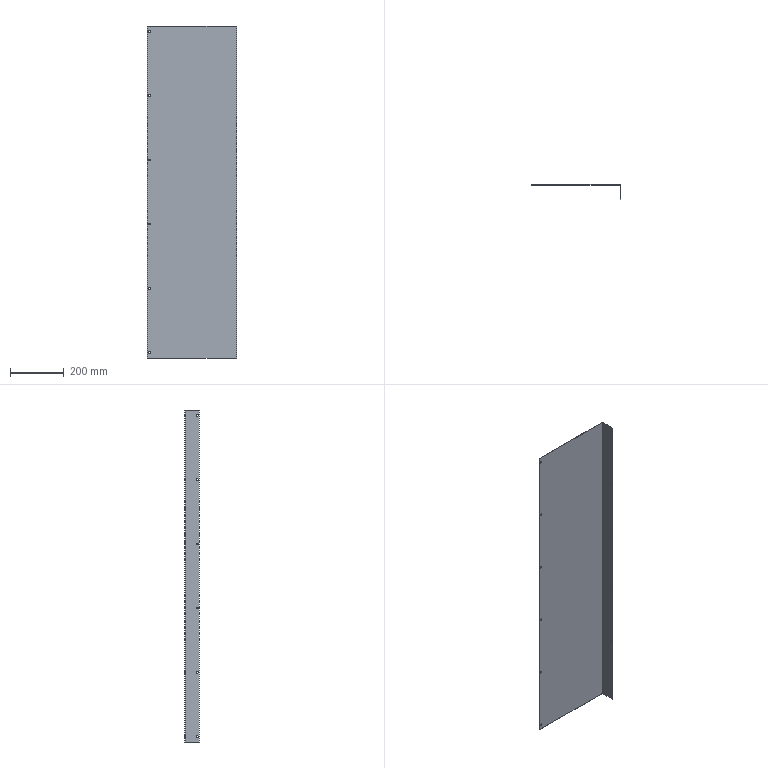Part | 1 solid | 74 faces | box 333.5 x 54 x 1240 mm | volume 478332 mm3 | cylinder 38 | plane 36 | commonest cylinder face diameters 6 x36 0.4 x1 2.4 x1